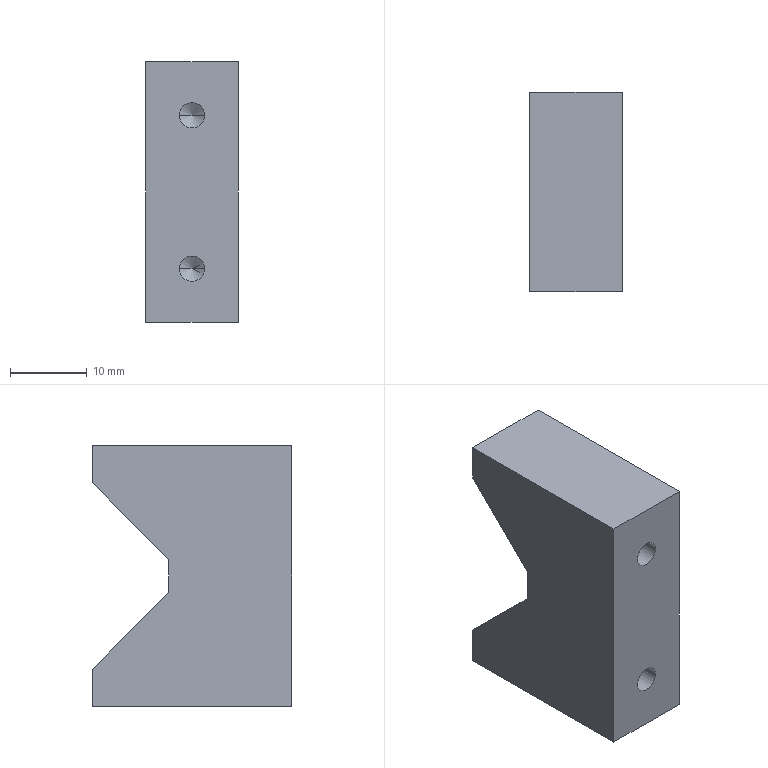Part | STEP file | 04-13 Guide block | 1 solid | 18 faces | box 12 x 26 x 34 mm | volume 8647 mm3 | plane 10 | cylinder 4 | cone 4 | commonest cylinder face diameters 3.3 x4
STEP:
#1=CARTESIAN_POINT('',(0.,0.,0.));
#2=DIRECTION('',(0.,0.,1.));
#3=DIRECTION('',(1.,0.,0.));
#4=AXIS2_PLACEMENT_3D('',#1,#2,#3);
#5=CARTESIAN_POINT('',(1.65,14.1,10.));
#6=VERTEX_POINT('',#5);
#7=CARTESIAN_POINT('',(1.65,0.,10.));
#8=VERTEX_POINT('',#7);
#9=CARTESIAN_POINT('',(1.65,14.1,10.));
#10=DIRECTION('',(0.,-1.,0.));
#11=VECTOR('',#10,1.);
#12=LINE('',#9,#11);
#13=CARTESIAN_POINT('',(0.,14.1,10.));
#14=DIRECTION('',(0.,-1.,0.));
#15=DIRECTION('',(1.,0.,0.));
#16=AXIS2_PLACEMENT_3D('',#13,#14,#15);
#17=CYLINDRICAL_SURFACE('',#16,1.65);
#18=CARTESIAN_POINT('',(6.283,0.));
#19=DIRECTION('',(0.,1.));
#20=VECTOR('',#19,1.);
#21=LINE('',#18,#20);
#22=(GEOMETRIC_REPRESENTATION_CONTEXT(2)PARAMETRIC_REPRESENTATION_CONTEXT()REPRESENTATION_CONTEXT('',''));
#23=DEFINITIONAL_REPRESENTATION('',(#21),#22);
#24=PCURVE('',#17,#23);
#25=CARTESIAN_POINT('',(0.,14.1,10.));
#26=DIRECTION('',(0.,-1.,0.));
#27=DIRECTION('',(1.,0.,0.));
#28=AXIS2_PLACEMENT_3D('',#25,#26,#27);
#29=CYLINDRICAL_SURFACE('',#28,1.65);
#30=CARTESIAN_POINT('',(0.,0.));
#31=DIRECTION('',(0.,1.));
#32=VECTOR('',#31,1.);
#33=LINE('',#30,#32);
#34=(GEOMETRIC_REPRESENTATION_CONTEXT(2)PARAMETRIC_REPRESENTATION_CONTEXT()REPRESENTATION_CONTEXT('',''));
#35=DEFINITIONAL_REPRESENTATION('',(#33),#34);
#36=PCURVE('',#29,#35);
#37=SURFACE_CURVE('',#12,(#24,#36),.PCURVE_S1.);
#38=EDGE_CURVE('',#6,#8,#37,.T.);
#39=ORIENTED_EDGE('',*,*,#38,.T.);
#40=CARTESIAN_POINT('',(-1.65,0.,10.));
#41=VERTEX_POINT('',#40);
#42=CARTESIAN_POINT('',(0.,0.,10.));
#43=DIRECTION('',(0.,-1.,0.));
#44=DIRECTION('',(1.,0.,0.));
#45=AXIS2_PLACEMENT_3D('',#42,#43,#44);
#46=CIRCLE('',#45,1.65);
#47=CARTESIAN_POINT('',(0.,14.1));
#48=DIRECTION('',(1.,0.));
#49=VECTOR('',#48,1.);
#50=LINE('',#47,#49);
#51=(GEOMETRIC_REPRESENTATION_CONTEXT(2)PARAMETRIC_REPRESENTATION_CONTEXT()REPRESENTATION_CONTEXT('',''));
#52=DEFINITIONAL_REPRESENTATION('',(#50),#51);
#53=PCURVE('',#17,#52);
#54=CARTESIAN_POINT('',(-6.,0.,-17.));
#55=DIRECTION('',(0.,1.,0.));
#56=DIRECTION('',(0.,0.,1.));
#57=AXIS2_PLACEMENT_3D('',#54,#55,#56);
#58=PLANE('',#57);
#59=CARTESIAN_POINT('',(27.,7.65));
#60=CARTESIAN_POINT('',(29.858,7.65));
#61=CARTESIAN_POINT('',(28.429,5.175));
#62=CARTESIAN_POINT('',(27.,2.7));
#63=CARTESIAN_POINT('',(25.571,5.175));
#64=CARTESIAN_POINT('',(24.142,7.65));
#65=CARTESIAN_POINT('',(27.,7.65));
#66=(BOUNDED_CURVE()B_SPLINE_CURVE(2,(#59,#60,#61,#62,#63,#64,#65),.UNSPECIFIED.,.T.,.F.)B_SPLINE_CURVE_WITH_KNOTS((1,2,2,2,2,1),(-2.094,0.,2.094,4.189,6.283,8.378),.UNSPECIFIED.)CURVE()GEOMETRIC_REPRESENTATION_ITEM()RATIONAL_B_SPLINE_CURVE((1.,0.5,1.,0.5,1.,0.5,1.))REPRESENTATION_ITEM(''));
#67=(GEOMETRIC_REPRESENTATION_CONTEXT(2)PARAMETRIC_REPRESENTATION_CONTEXT()REPRESENTATION_CONTEXT('',''));
#68=DEFINITIONAL_REPRESENTATION('',(#66),#67);
#69=PCURVE('',#58,#68);
#70=SURFACE_CURVE('',#46,(#53,#69),.PCURVE_S1.);
#71=EDGE_CURVE('',#41,#8,#70,.T.);
#72=ORIENTED_EDGE('',*,*,#71,.F.);
#73=CARTESIAN_POINT('',(-1.65,14.1,10.));
#74=VERTEX_POINT('',#73);
#75=CARTESIAN_POINT('',(-1.65,14.1,10.));
#76=DIRECTION('',(0.,-1.,0.));
#77=VECTOR('',#76,1.);
#78=LINE('',#75,#77);
#79=CARTESIAN_POINT('',(3.142,0.));
#80=DIRECTION('',(0.,1.));
#81=VECTOR('',#80,1.);
#82=LINE('',#79,#81);
#83=(GEOMETRIC_REPRESENTATION_CONTEXT(2)PARAMETRIC_REPRESENTATION_CONTEXT()REPRESENTATION_CONTEXT('',''));
#84=DEFINITIONAL_REPRESENTATION('',(#82),#83);
#85=PCURVE('',#17,#84);
#86=CARTESIAN_POINT('',(3.142,0.));
#87=DIRECTION('',(0.,1.));
#88=VECTOR('',#87,1.);
#89=LINE('',#86,#88);
#90=(GEOMETRIC_REPRESENTATION_CONTEXT(2)PARAMETRIC_REPRESENTATION_CONTEXT()REPRESENTATION_CONTEXT('',''));
#91=DEFINITIONAL_REPRESENTATION('',(#89),#90);
#92=PCURVE('',#29,#91);
#93=SURFACE_CURVE('',#78,(#85,#92),.PCURVE_S1.);
#94=EDGE_CURVE('',#74,#41,#93,.T.);
#95=ORIENTED_EDGE('',*,*,#94,.F.);
#96=CARTESIAN_POINT('',(0.,14.1,10.));
#97=DIRECTION('',(0.,1.,0.));
#98=DIRECTION('',(0.,0.,-1.));
#99=AXIS2_PLACEMENT_3D('',#96,#97,#98);
#100=CIRCLE('',#99,1.65);
#101=CARTESIAN_POINT('',(10.996,0.));
#102=DIRECTION('',(-1.,0.));
#103=VECTOR('',#102,1.);
#104=LINE('',#101,#103);
#105=(GEOMETRIC_REPRESENTATION_CONTEXT(2)PARAMETRIC_REPRESENTATION_CONTEXT()REPRESENTATION_CONTEXT('',''));
#106=DEFINITIONAL_REPRESENTATION('',(#104),#105);
#107=PCURVE('',#17,#106);
#108=CARTESIAN_POINT('',(0.,-984.909,10.));
#109=DIRECTION('',(0.,-1.,0.));
#110=DIRECTION('',(1.,0.,0.));
#111=AXIS2_PLACEMENT_3D('',#108,#109,#110);
#112=CONICAL_SURFACE('',#111,1664.279,1.03);
#113=CARTESIAN_POINT('',(10.996,-999.009));
#114=DIRECTION('',(-1.,0.));
#115=VECTOR('',#114,1.);
#116=LINE('',#113,#115);
#117=(GEOMETRIC_REPRESENTATION_CONTEXT(2)PARAMETRIC_REPRESENTATION_CONTEXT()REPRESENTATION_CONTEXT('',''));
#118=DEFINITIONAL_REPRESENTATION('',(#116),#117);
#119=PCURVE('',#112,#118);
#120=SURFACE_CURVE('',#100,(#107,#119),.PCURVE_S1.);
#121=EDGE_CURVE('',#6,#74,#120,.T.);
#122=ORIENTED_EDGE('',*,*,#121,.F.);
#123=EDGE_LOOP('',(#39,#72,#95,#122));
#124=FACE_BOUND('',#123,.F.);
#125=ADVANCED_FACE('',(#124),#17,.F.);
#126=ORIENTED_EDGE('',*,*,#121,.T.);
#127=CARTESIAN_POINT('',(0.,15.091,10.));
#128=VERTEX_POINT('',#127);
#129=CARTESIAN_POINT('',(0.,15.091,10.));
#130=DIRECTION('',(-0.8572,-0.515,0.));
#131=VECTOR('',#130,1.);
#132=LINE('',#129,#131);
#133=CARTESIAN_POINT('',(3.142,-1000.));
#134=CARTESIAN_POINT('',(3.142,-999.985));
#135=CARTESIAN_POINT('',(3.142,-999.955));
#136=CARTESIAN_POINT('',(3.142,-999.91));
#137=CARTESIAN_POINT('',(3.142,-999.865));
#138=CARTESIAN_POINT('',(3.142,-999.82));
#139=CARTESIAN_POINT('',(3.142,-999.775));
#140=CARTESIAN_POINT('',(3.142,-999.73));
#141=CARTESIAN_POINT('',(3.142,-999.685));
#142=CARTESIAN_POINT('',(3.142,-999.639));
#143=CARTESIAN_POINT('',(3.142,-999.594));
#144=CARTESIAN_POINT('',(3.142,-999.549));
#145=CARTESIAN_POINT('',(3.142,-999.504));
#146=CARTESIAN_POINT('',(3.142,-999.459));
#147=CARTESIAN_POINT('',(3.142,-999.414));
#148=CARTESIAN_POINT('',(3.142,-999.369));
#149=CARTESIAN_POINT('',(3.142,-999.324));
#150=CARTESIAN_POINT('',(3.142,-999.279));
#151=CARTESIAN_POINT('',(3.142,-999.234));
#152=CARTESIAN_POINT('',(3.142,-999.189));
#153=CARTESIAN_POINT('',(3.142,-999.144));
#154=CARTESIAN_POINT('',(3.142,-999.099));
#155=CARTESIAN_POINT('',(3.142,-999.054));
#156=CARTESIAN_POINT('',(3.142,-999.024));
#157=CARTESIAN_POINT('',(3.142,-999.009));
#158=B_SPLINE_CURVE_WITH_KNOTS('',3,(#133,#134,#135,#136,#137,#138,#139,#140,#141,#142,#143,#144,#145,#146,#147,#148,#149,#150,#151,#152,#153,#154,#155,#156,#157),.UNSPECIFIED.,.F.,.F.,(4,1,1,1,1,1,1,1,1,1,1,1,1,1,1,1,1,1,1,1,1,1,4),(0.,0.0875,0.175,0.2625,0.35,0.4375,0.525,0.6125,0.7,0.7875,0.875,0.9625,1.05,1.137,1.225,1.312,1.4,1.487,1.575,1.662,1.75,1.837,1.925),.QUASI_UNIFORM_KNOTS.);
#159=(GEOMETRIC_REPRESENTATION_CONTEXT(2)PARAMETRIC_REPRESENTATION_CONTEXT()REPRESENTATION_CONTEXT('',''));
#160=DEFINITIONAL_REPRESENTATION('',(#158),#159);
#161=PCURVE('',#112,#160);
#162=CARTESIAN_POINT('',(0.,-984.909,10.));
#163=DIRECTION('',(0.,-1.,0.));
#164=DIRECTION('',(1.,0.,0.));
#165=AXIS2_PLACEMENT_3D('',#162,#163,#164);
#166=CONICAL_SURFACE('',#165,1664.279,1.03);
#167=CARTESIAN_POINT('',(3.142,-1000.));
#168=CARTESIAN_POINT('',(3.142,-999.985));
#169=CARTESIAN_POINT('',(3.142,-999.955));
#170=CARTESIAN_POINT('',(3.142,-999.91));
#171=CARTESIAN_POINT('',(3.142,-999.865));
#172=CARTESIAN_POINT('',(3.142,-999.82));
#173=CARTESIAN_POINT('',(3.142,-999.775));
#174=CARTESIAN_POINT('',(3.142,-999.73));
#175=CARTESIAN_POINT('',(3.142,-999.685));
#176=CARTESIAN_POINT('',(3.142,-999.639));
#177=CARTESIAN_POINT('',(3.142,-999.594));
#178=CARTESIAN_POINT('',(3.142,-999.549));
#179=CARTESIAN_POINT('',(3.142,-999.504));
#180=CARTESIAN_POINT('',(3.142,-999.459));
#181=CARTESIAN_POINT('',(3.142,-999.414));
#182=CARTESIAN_POINT('',(3.142,-999.369));
#183=CARTESIAN_POINT('',(3.142,-999.324));
#184=CARTESIAN_POINT('',(3.142,-999.279));
#185=CARTESIAN_POINT('',(3.142,-999.234));
#186=CARTESIAN_POINT('',(3.142,-999.189));
#187=CARTESIAN_POINT('',(3.142,-999.144));
#188=CARTESIAN_POINT('',(3.142,-999.099));
#189=CARTESIAN_POINT('',(3.142,-999.054));
#190=CARTESIAN_POINT('',(3.142,-999.024));
#191=CARTESIAN_POINT('',(3.142,-999.009));
#192=B_SPLINE_CURVE_WITH_KNOTS('',3,(#167,#168,#169,#170,#171,#172,#173,#174,#175,#176,#177,#178,#179,#180,#181,#182,#183,#184,#185,#186,#187,#188,#189,#190,#191),.UNSPECIFIED.,.F.,.F.,(4,1,1,1,1,1,1,1,1,1,1,1,1,1,1,1,1,1,1,1,1,1,4),(0.,0.0875,0.175,0.2625,0.35,0.4375,0.525,0.6125,0.7,0.7875,0.875,0.9625,1.05,1.137,1.225,1.312,1.4,1.487,1.575,1.662,1.75,1.837,1.925),.QUASI_UNIFORM_KNOTS.);
#193=(GEOMETRIC_REPRESENTATION_CONTEXT(2)PARAMETRIC_REPRESENTATION_CONTEXT()REPRESENTATION_CONTEXT('',''));
#194=DEFINITIONAL_REPRESENTATION('',(#192),#193);
#195=PCURVE('',#166,#194);
#196=SURFACE_CURVE('',#132,(#161,#195),.PCURVE_S1.);
#197=EDGE_CURVE('',#128,#74,#196,.T.);
#198=ORIENTED_EDGE('',*,*,#197,.F.);
#199=CARTESIAN_POINT('',(0.,15.091,10.));
#200=DIRECTION('',(0.8572,-0.515,0.));
#201=VECTOR('',#200,1.);
#202=LINE('',#199,#201);
#203=CARTESIAN_POINT('',(6.283,-1000.));
#204=DIRECTION('',(0.,1.));
#205=VECTOR('',#204,1.);
#206=LINE('',#203,#205);
#207=(GEOMETRIC_REPRESENTATION_CONTEXT(2)PARAMETRIC_REPRESENTATION_CONTEXT()REPRESENTATION_CONTEXT('',''));
#208=DEFINITIONAL_REPRESENTATION('',(#206),#207);
#209=PCURVE('',#112,#208);
#210=CARTESIAN_POINT('',(0.,-1000.));
#211=DIRECTION('',(0.,1.));
#212=VECTOR('',#211,1.);
#213=LINE('',#210,#212);
#214=(GEOMETRIC_REPRESENTATION_CONTEXT(2)PARAMETRIC_REPRESENTATION_CONTEXT()REPRESENTATION_CONTEXT('',''));
#215=DEFINITIONAL_REPRESENTATION('',(#213),#214);
#216=PCURVE('',#166,#215);
#217=SURFACE_CURVE('',#202,(#209,#216),.PCURVE_S1.);
#218=EDGE_CURVE('',#128,#6,#217,.T.);
#219=ORIENTED_EDGE('',*,*,#218,.T.);
#220=EDGE_LOOP('',(#126,#198,#219));
#221=FACE_BOUND('',#220,.F.);
#222=ADVANCED_FACE('',(#221),#112,.F.);
#223=CARTESIAN_POINT('',(1.65,14.1,-10.));
#224=VERTEX_POINT('',#223);
#225=CARTESIAN_POINT('',(1.65,0.,-10.));
#226=VERTEX_POINT('',#225);
#227=CARTESIAN_POINT('',(1.65,14.1,-10.));
#228=DIRECTION('',(0.,-1.,0.));
#229=VECTOR('',#228,1.);
#230=LINE('',#227,#229);
#231=CARTESIAN_POINT('',(0.,14.1,-10.));
#232=DIRECTION('',(0.,-1.,0.));
#233=DIRECTION('',(1.,0.,0.));
#234=AXIS2_PLACEMENT_3D('',#231,#232,#233);
#235=CYLINDRICAL_SURFACE('',#234,1.65);
#236=CARTESIAN_POINT('',(6.283,0.));
#237=DIRECTION('',(0.,1.));
#238=VECTOR('',#237,1.);
#239=LINE('',#236,#238);
#240=(GEOMETRIC_REPRESENTATION_CONTEXT(2)PARAMETRIC_REPRESENTATION_CONTEXT()REPRESENTATION_CONTEXT('',''));
#241=DEFINITIONAL_REPRESENTATION('',(#239),#240);
#242=PCURVE('',#235,#241);
#243=CARTESIAN_POINT('',(0.,14.1,-10.));
#244=DIRECTION('',(0.,-1.,0.));
#245=DIRECTION('',(1.,0.,0.));
#246=AXIS2_PLACEMENT_3D('',#243,#244,#245);
#247=CYLINDRICAL_SURFACE('',#246,1.65);
#248=CARTESIAN_POINT('',(0.,0.));
#249=DIRECTION('',(0.,1.));
#250=VECTOR('',#249,1.);
#251=LINE('',#248,#250);
#252=(GEOMETRIC_REPRESENTATION_CONTEXT(2)PARAMETRIC_REPRESENTATION_CONTEXT()REPRESENTATION_CONTEXT('',''));
#253=DEFINITIONAL_REPRESENTATION('',(#251),#252);
#254=PCURVE('',#247,#253);
#255=SURFACE_CURVE('',#230,(#242,#254),.PCURVE_S1.);
#256=EDGE_CURVE('',#224,#226,#255,.T.);
#257=ORIENTED_EDGE('',*,*,#256,.T.);
#258=CARTESIAN_POINT('',(-1.65,0.,-10.));
#259=VERTEX_POINT('',#258);
#260=CARTESIAN_POINT('',(0.,0.,-10.));
#261=DIRECTION('',(0.,-1.,0.));
#262=DIRECTION('',(1.,0.,0.));
#263=AXIS2_PLACEMENT_3D('',#260,#261,#262);
#264=CIRCLE('',#263,1.65);
#265=CARTESIAN_POINT('',(0.,14.1));
#266=DIRECTION('',(1.,0.));
#267=VECTOR('',#266,1.);
#268=LINE('',#265,#267);
#269=(GEOMETRIC_REPRESENTATION_CONTEXT(2)PARAMETRIC_REPRESENTATION_CONTEXT()REPRESENTATION_CONTEXT('',''));
#270=DEFINITIONAL_REPRESENTATION('',(#268),#269);
#271=PCURVE('',#235,#270);
#272=CARTESIAN_POINT('',(7.,7.65));
#273=CARTESIAN_POINT('',(9.858,7.65));
#274=CARTESIAN_POINT('',(8.429,5.175));
#275=CARTESIAN_POINT('',(7.,2.7));
#276=CARTESIAN_POINT('',(5.571,5.175));
#277=CARTESIAN_POINT('',(4.142,7.65));
#278=CARTESIAN_POINT('',(7.,7.65));
#279=(BOUNDED_CURVE()B_SPLINE_CURVE(2,(#272,#273,#274,#275,#276,#277,#278),.UNSPECIFIED.,.T.,.F.)B_SPLINE_CURVE_WITH_KNOTS((1,2,2,2,2,1),(-2.094,0.,2.094,4.189,6.283,8.378),.UNSPECIFIED.)CURVE()GEOMETRIC_REPRESENTATION_ITEM()RATIONAL_B_SPLINE_CURVE((1.,0.5,1.,0.5,1.,0.5,1.))REPRESENTATION_ITEM(''));
#280=(GEOMETRIC_REPRESENTATION_CONTEXT(2)PARAMETRIC_REPRESENTATION_CONTEXT()REPRESENTATION_CONTEXT('',''));
#281=DEFINITIONAL_REPRESENTATION('',(#279),#280);
#282=PCURVE('',#58,#281);
#283=SURFACE_CURVE('',#264,(#271,#282),.PCURVE_S1.);
#284=EDGE_CURVE('',#259,#226,#283,.T.);
#285=ORIENTED_EDGE('',*,*,#284,.F.);
#286=CARTESIAN_POINT('',(-1.65,14.1,-10.));
#287=VERTEX_POINT('',#286);
#288=CARTESIAN_POINT('',(-1.65,14.1,-10.));
#289=DIRECTION('',(0.,-1.,0.));
#290=VECTOR('',#289,1.);
#291=LINE('',#288,#290);
#292=CARTESIAN_POINT('',(3.142,0.));
#293=DIRECTION('',(0.,1.));
#294=VECTOR('',#293,1.);
#295=LINE('',#292,#294);
#296=(GEOMETRIC_REPRESENTATION_CONTEXT(2)PARAMETRIC_REPRESENTATION_CONTEXT()REPRESENTATION_CONTEXT('',''));
#297=DEFINITIONAL_REPRESENTATION('',(#295),#296);
#298=PCURVE('',#235,#297);
#299=CARTESIAN_POINT('',(3.142,0.));
#300=DIRECTION('',(0.,1.));
#301=VECTOR('',#300,1.);
#302=LINE('',#299,#301);
#303=(GEOMETRIC_REPRESENTATION_CONTEXT(2)PARAMETRIC_REPRESENTATION_CONTEXT()REPRESENTATION_CONTEXT('',''));
#304=DEFINITIONAL_REPRESENTATION('',(#302),#303);
#305=PCURVE('',#247,#304);
#306=SURFACE_CURVE('',#291,(#298,#305),.PCURVE_S1.);
#307=EDGE_CURVE('',#287,#259,#306,.T.);
#308=ORIENTED_EDGE('',*,*,#307,.F.);
#309=CARTESIAN_POINT('',(0.,14.1,-10.));
#310=DIRECTION('',(0.,1.,0.));
#311=DIRECTION('',(0.,0.,-1.));
#312=AXIS2_PLACEMENT_3D('',#309,#310,#311);
#313=CIRCLE('',#312,1.65);
#314=CARTESIAN_POINT('',(10.996,0.));
#315=DIRECTION('',(-1.,0.));
#316=VECTOR('',#315,1.);
#317=LINE('',#314,#316);
#318=(GEOMETRIC_REPRESENTATION_CONTEXT(2)PARAMETRIC_REPRESENTATION_CONTEXT()REPRESENTATION_CONTEXT('',''));
#319=DEFINITIONAL_REPRESENTATION('',(#317),#318);
#320=PCURVE('',#235,#319);
#321=CARTESIAN_POINT('',(0.,-984.909,-10.));
#322=DIRECTION('',(0.,-1.,0.));
#323=DIRECTION('',(1.,0.,0.));
#324=AXIS2_PLACEMENT_3D('',#321,#322,#323);
#325=CONICAL_SURFACE('',#324,1664.279,1.03);
#326=CARTESIAN_POINT('',(10.996,-999.009));
#327=DIRECTION('',(-1.,0.));
#328=VECTOR('',#327,1.);
#329=LINE('',#326,#328);
#330=(GEOMETRIC_REPRESENTATION_CONTEXT(2)PARAMETRIC_REPRESENTATION_CONTEXT()REPRESENTATION_CONTEXT('',''));
#331=DEFINITIONAL_REPRESENTATION('',(#329),#330);
#332=PCURVE('',#325,#331);
#333=SURFACE_CURVE('',#313,(#320,#332),.PCURVE_S1.);
#334=EDGE_CURVE('',#224,#287,#333,.T.);
#335=ORIENTED_EDGE('',*,*,#334,.F.);
#336=EDGE_LOOP('',(#257,#285,#308,#335));
#337=FACE_BOUND('',#336,.F.);
#338=ADVANCED_FACE('',(#337),#235,.F.);
#339=ORIENTED_EDGE('',*,*,#334,.T.);
#340=CARTESIAN_POINT('',(0.,15.091,-10.));
#341=VERTEX_POINT('',#340);
#342=CARTESIAN_POINT('',(0.,15.091,-10.));
#343=DIRECTION('',(-0.8572,-0.515,0.));
#344=VECTOR('',#343,1.);
#345=LINE('',#342,#344);
#346=CARTESIAN_POINT('',(3.142,-1000.));
#347=CARTESIAN_POINT('',(3.142,-999.985));
#348=CARTESIAN_POINT('',(3.142,-999.955));
#349=CARTESIAN_POINT('',(3.142,-999.91));
#350=CARTESIAN_POINT('',(3.142,-999.865));
#351=CARTESIAN_POINT('',(3.142,-999.82));
#352=CARTESIAN_POINT('',(3.142,-999.775));
#353=CARTESIAN_POINT('',(3.142,-999.73));
#354=CARTESIAN_POINT('',(3.142,-999.685));
#355=CARTESIAN_POINT('',(3.142,-999.639));
#356=CARTESIAN_POINT('',(3.142,-999.594));
#357=CARTESIAN_POINT('',(3.142,-999.549));
#358=CARTESIAN_POINT('',(3.142,-999.504));
#359=CARTESIAN_POINT('',(3.142,-999.459));
#360=CARTESIAN_POINT('',(3.142,-999.414));
#361=CARTESIAN_POINT('',(3.142,-999.369));
#362=CARTESIAN_POINT('',(3.142,-999.324));
#363=CARTESIAN_POINT('',(3.142,-999.279));
#364=CARTESIAN_POINT('',(3.142,-999.234));
#365=CARTESIAN_POINT('',(3.142,-999.189));
#366=CARTESIAN_POINT('',(3.142,-999.144));
#367=CARTESIAN_POINT('',(3.142,-999.099));
#368=CARTESIAN_POINT('',(3.142,-999.054));
#369=CARTESIAN_POINT('',(3.142,-999.024));
#370=CARTESIAN_POINT('',(3.142,-999.009));
#371=B_SPLINE_CURVE_WITH_KNOTS('',3,(#346,#347,#348,#349,#350,#351,#352,#353,#354,#355,#356,#357,#358,#359,#360,#361,#362,#363,#364,#365,#366,#367,#368,#369,#370),.UNSPECIFIED.,.F.,.F.,(4,1,1,1,1,1,1,1,1,1,1,1,1,1,1,1,1,1,1,1,1,1,4),(0.,0.0875,0.175,0.2625,0.35,0.4375,0.525,0.6125,0.7,0.7875,0.875,0.9625,1.05,1.137,1.225,1.312,1.4,1.487,1.575,1.662,1.75,1.837,1.925),.QUASI_UNIFORM_KNOTS.);
#372=(GEOMETRIC_REPRESENTATION_CONTEXT(2)PARAMETRIC_REPRESENTATION_CONTEXT()REPRESENTATION_CONTEXT('',''));
#373=DEFINITIONAL_REPRESENTATION('',(#371),#372);
#374=PCURVE('',#325,#373);
#375=CARTESIAN_POINT('',(0.,-984.909,-10.));
#376=DIRECTION('',(0.,-1.,0.));
#377=DIRECTION('',(1.,0.,0.));
#378=AXIS2_PLACEMENT_3D('',#375,#376,#377);
#379=CONICAL_SURFACE('',#378,1664.279,1.03);
#380=CARTESIAN_POINT('',(3.142,-1000.));
#381=CARTESIAN_POINT('',(3.142,-999.985));
#382=CARTESIAN_POINT('',(3.142,-999.955));
#383=CARTESIAN_POINT('',(3.142,-999.91));
#384=CARTESIAN_POINT('',(3.142,-999.865));
#385=CARTESIAN_POINT('',(3.142,-999.82));
#386=CARTESIAN_POINT('',(3.142,-999.775));
#387=CARTESIAN_POINT('',(3.142,-999.73));
#388=CARTESIAN_POINT('',(3.142,-999.685));
#389=CARTESIAN_POINT('',(3.142,-999.639));
#390=CARTESIAN_POINT('',(3.142,-999.594));
#391=CARTESIAN_POINT('',(3.142,-999.549));
#392=CARTESIAN_POINT('',(3.142,-999.504));
#393=CARTESIAN_POINT('',(3.142,-999.459));
#394=CARTESIAN_POINT('',(3.142,-999.414));
#395=CARTESIAN_POINT('',(3.142,-999.369));
#396=CARTESIAN_POINT('',(3.142,-999.324));
#397=CARTESIAN_POINT('',(3.142,-999.279));
#398=CARTESIAN_POINT('',(3.142,-999.234));
#399=CARTESIAN_POINT('',(3.142,-999.189));
#400=CARTESIAN_POINT('',(3.142,-999.144));
#401=CARTESIAN_POINT('',(3.142,-999.099));
#402=CARTESIAN_POINT('',(3.142,-999.054));
#403=CARTESIAN_POINT('',(3.142,-999.024));
#404=CARTESIAN_POINT('',(3.142,-999.009));
#405=B_SPLINE_CURVE_WITH_KNOTS('',3,(#380,#381,#382,#383,#384,#385,#386,#387,#388,#389,#390,#391,#392,#393,#394,#395,#396,#397,#398,#399,#400,#401,#402,#403,#404),.UNSPECIFIED.,.F.,.F.,(4,1,1,1,1,1,1,1,1,1,1,1,1,1,1,1,1,1,1,1,1,1,4),(0.,0.0875,0.175,0.2625,0.35,0.4375,0.525,0.6125,0.7,0.7875,0.875,0.9625,1.05,1.137,1.225,1.312,1.4,1.487,1.575,1.662,1.75,1.837,1.925),.QUASI_UNIFORM_KNOTS.);
#406=(GEOMETRIC_REPRESENTATION_CONTEXT(2)PARAMETRIC_REPRESENTATION_CONTEXT()REPRESENTATION_CONTEXT('',''));
#407=DEFINITIONAL_REPRESENTATION('',(#405),#406);
#408=PCURVE('',#379,#407);
#409=SURFACE_CURVE('',#345,(#374,#408),.PCURVE_S1.);
#410=EDGE_CURVE('',#341,#287,#409,.T.);
#411=ORIENTED_EDGE('',*,*,#410,.F.);
#412=CARTESIAN_POINT('',(0.,15.091,-10.));
#413=DIRECTION('',(0.8572,-0.515,0.));
#414=VECTOR('',#413,1.);
#415=LINE('',#412,#414);
#416=CARTESIAN_POINT('',(6.283,-1000.));
#417=DIRECTION('',(0.,1.));
#418=VECTOR('',#417,1.);
#419=LINE('',#416,#418);
#420=(GEOMETRIC_REPRESENTATION_CONTEXT(2)PARAMETRIC_REPRESENTATION_CONTEXT()REPRESENTATION_CONTEXT('',''));
#421=DEFINITIONAL_REPRESENTATION('',(#419),#420);
#422=PCURVE('',#325,#421);
#423=CARTESIAN_POINT('',(0.,-1000.));
#424=DIRECTION('',(0.,1.));
#425=VECTOR('',#424,1.);
#426=LINE('',#423,#425);
#427=(GEOMETRIC_REPRESENTATION_CONTEXT(2)PARAMETRIC_REPRESENTATION_CONTEXT()REPRESENTATION_CONTEXT('',''));
#428=DEFINITIONAL_REPRESENTATION('',(#426),#427);
#429=PCURVE('',#379,#428);
#430=SURFACE_CURVE('',#415,(#422,#429),.PCURVE_S1.);
#431=EDGE_CURVE('',#341,#224,#430,.T.);
#432=ORIENTED_EDGE('',*,*,#431,.T.);
#433=EDGE_LOOP('',(#339,#411,#432));
#434=FACE_BOUND('',#433,.F.);
#435=ADVANCED_FACE('',(#434),#325,.F.);
#436=CARTESIAN_POINT('',(0.,0.,10.));
#437=DIRECTION('',(0.,-1.,0.));
#438=DIRECTION('',(1.,0.,0.));
#439=AXIS2_PLACEMENT_3D('',#436,#437,#438);
#440=CIRCLE('',#439,1.65);
#441=CARTESIAN_POINT('',(0.,14.1));
#442=DIRECTION('',(1.,0.));
#443=VECTOR('',#442,1.);
#444=LINE('',#441,#443);
#445=(GEOMETRIC_REPRESENTATION_CONTEXT(2)PARAMETRIC_REPRESENTATION_CONTEXT()REPRESENTATION_CONTEXT('',''));
#446=DEFINITIONAL_REPRESENTATION('',(#444),#445);
#447=PCURVE('',#29,#446);
#448=CARTESIAN_POINT('',(27.,7.65));
#449=CARTESIAN_POINT('',(29.858,7.65));
#450=CARTESIAN_POINT('',(28.429,5.175));
#451=CARTESIAN_POINT('',(27.,2.7));
#452=CARTESIAN_POINT('',(25.571,5.175));
#453=CARTESIAN_POINT('',(24.142,7.65));
#454=CARTESIAN_POINT('',(27.,7.65));
#455=(BOUNDED_CURVE()B_SPLINE_CURVE(2,(#448,#449,#450,#451,#452,#453,#454),.UNSPECIFIED.,.T.,.F.)B_SPLINE_CURVE_WITH_KNOTS((1,2,2,2,2,1),(-2.094,0.,2.094,4.189,6.283,8.378),.UNSPECIFIED.)CURVE()GEOMETRIC_REPRESENTATION_ITEM()RATIONAL_B_SPLINE_CURVE((1.,0.5,1.,0.5,1.,0.5,1.))REPRESENTATION_ITEM(''));
#456=(GEOMETRIC_REPRESENTATION_CONTEXT(2)PARAMETRIC_REPRESENTATION_CONTEXT()REPRESENTATION_CONTEXT('',''));
#457=DEFINITIONAL_REPRESENTATION('',(#455),#456);
#458=PCURVE('',#58,#457);
#459=SURFACE_CURVE('',#440,(#447,#458),.PCURVE_S1.);
#460=EDGE_CURVE('',#8,#41,#459,.T.);
#461=ORIENTED_EDGE('',*,*,#460,.F.);
#462=ORIENTED_EDGE('',*,*,#38,.F.);
#463=CARTESIAN_POINT('',(0.,14.1,10.));
#464=DIRECTION('',(0.,1.,0.));
#465=DIRECTION('',(0.,0.,-1.));
#466=AXIS2_PLACEMENT_3D('',#463,#464,#465);
#467=CIRCLE('',#466,1.65);
#468=CARTESIAN_POINT('',(4.712,0.));
#469=DIRECTION('',(-1.,0.));
#470=VECTOR('',#469,1.);
#471=LINE('',#468,#470);
#472=(GEOMETRIC_REPRESENTATION_CONTEXT(2)PARAMETRIC_REPRESENTATION_CONTEXT()REPRESENTATION_CONTEXT('',''));
#473=DEFINITIONAL_REPRESENTATION('',(#471),#472);
#474=PCURVE('',#29,#473);
#475=CARTESIAN_POINT('',(4.712,-999.009));
#476=DIRECTION('',(-1.,0.));
#477=VECTOR('',#476,1.);
#478=LINE('',#475,#477);
#479=(GEOMETRIC_REPRESENTATION_CONTEXT(2)PARAMETRIC_REPRESENTATION_CONTEXT()REPRESENTATION_CONTEXT('',''));
#480=DEFINITIONAL_REPRESENTATION('',(#478),#479);
#481=PCURVE('',#166,#480);
#482=SURFACE_CURVE('',#467,(#474,#481),.PCURVE_S1.);
#483=EDGE_CURVE('',#74,#6,#482,.T.);
#484=ORIENTED_EDGE('',*,*,#483,.F.);
#485=ORIENTED_EDGE('',*,*,#94,.T.);
#486=EDGE_LOOP('',(#461,#462,#484,#485));
#487=FACE_BOUND('',#486,.F.);
#488=ADVANCED_FACE('',(#487),#29,.F.);
#489=CARTESIAN_POINT('',(0.,0.,-10.));
#490=DIRECTION('',(0.,-1.,0.));
#491=DIRECTION('',(1.,0.,0.));
#492=AXIS2_PLACEMENT_3D('',#489,#490,#491);
#493=CIRCLE('',#492,1.65);
#494=CARTESIAN_POINT('',(7.,7.65));
#495=CARTESIAN_POINT('',(9.858,7.65));
#496=CARTESIAN_POINT('',(8.429,5.175));
#497=CARTESIAN_POINT('',(7.,2.7));
#498=CARTESIAN_POINT('',(5.571,5.175));
#499=CARTESIAN_POINT('',(4.142,7.65));
#500=CARTESIAN_POINT('',(7.,7.65));
#501=(BOUNDED_CURVE()B_SPLINE_CURVE(2,(#494,#495,#496,#497,#498,#499,#500),.UNSPECIFIED.,.T.,.F.)B_SPLINE_CURVE_WITH_KNOTS((1,2,2,2,2,1),(-2.094,0.,2.094,4.189,6.283,8.378),.UNSPECIFIED.)CURVE()GEOMETRIC_REPRESENTATION_ITEM()RATIONAL_B_SPLINE_CURVE((1.,0.5,1.,0.5,1.,0.5,1.))REPRESENTATION_ITEM(''));
#502=(GEOMETRIC_REPRESENTATION_CONTEXT(2)PARAMETRIC_REPRESENTATION_CONTEXT()REPRESENTATION_CONTEXT('',''));
#503=DEFINITIONAL_REPRESENTATION('',(#501),#502);
#504=PCURVE('',#58,#503);
#505=CARTESIAN_POINT('',(0.,14.1));
#506=DIRECTION('',(1.,0.));
#507=VECTOR('',#506,1.);
#508=LINE('',#505,#507);
#509=(GEOMETRIC_REPRESENTATION_CONTEXT(2)PARAMETRIC_REPRESENTATION_CONTEXT()REPRESENTATION_CONTEXT('',''));
#510=DEFINITIONAL_REPRESENTATION('',(#508),#509);
#511=PCURVE('',#247,#510);
#512=SURFACE_CURVE('',#493,(#504,#511),.PCURVE_S1.);
#513=EDGE_CURVE('',#226,#259,#512,.T.);
#514=ORIENTED_EDGE('',*,*,#513,.F.);
#515=ORIENTED_EDGE('',*,*,#284,.F.);
#516=EDGE_LOOP('',(#514,#515));
#517=FACE_BOUND('',#516,.T.);
#518=ORIENTED_EDGE('',*,*,#460,.F.);
#519=ORIENTED_EDGE('',*,*,#71,.F.);
#520=EDGE_LOOP('',(#518,#519));
#521=FACE_BOUND('',#520,.T.);
#522=CARTESIAN_POINT('',(6.,0.,-17.));
#523=VERTEX_POINT('',#522);
#524=CARTESIAN_POINT('',(-6.,0.,-17.));
#525=VERTEX_POINT('',#524);
#526=CARTESIAN_POINT('',(0.,0.,-17.));
#527=DIRECTION('',(-1.,0.,0.));
#528=VECTOR('',#527,1.);
#529=LINE('',#526,#528);
#530=CARTESIAN_POINT('',(0.,6.));
#531=DIRECTION('',(0.,-1.));
#532=VECTOR('',#531,1.);
#533=LINE('',#530,#532);
#534=(GEOMETRIC_REPRESENTATION_CONTEXT(2)PARAMETRIC_REPRESENTATION_CONTEXT()REPRESENTATION_CONTEXT('',''));
#535=DEFINITIONAL_REPRESENTATION('',(#533),#534);
#536=PCURVE('',#58,#535);
#537=CARTESIAN_POINT('',(-6.,0.,-17.));
#538=DIRECTION('',(0.,0.,1.));
#539=DIRECTION('',(1.,0.,0.));
#540=AXIS2_PLACEMENT_3D('',#537,#538,#539);
#541=PLANE('',#540);
#542=CARTESIAN_POINT('',(6.,0.));
#543=DIRECTION('',(-1.,0.));
#544=VECTOR('',#543,1.);
#545=LINE('',#542,#544);
#546=(GEOMETRIC_REPRESENTATION_CONTEXT(2)PARAMETRIC_REPRESENTATION_CONTEXT()REPRESENTATION_CONTEXT('',''));
#547=DEFINITIONAL_REPRESENTATION('',(#545),#546);
#548=PCURVE('',#541,#547);
#549=SURFACE_CURVE('',#529,(#536,#548),.PCURVE_S1.);
#550=EDGE_CURVE('',#523,#525,#549,.T.);
#551=ORIENTED_EDGE('',*,*,#550,.F.);
#552=CARTESIAN_POINT('',(6.,0.,17.));
#553=VERTEX_POINT('',#552);
#554=CARTESIAN_POINT('',(6.,0.,0.));
#555=DIRECTION('',(0.,0.,-1.));
#556=VECTOR('',#555,1.);
#557=LINE('',#554,#556);
#558=CARTESIAN_POINT('',(17.,12.));
#559=DIRECTION('',(-1.,0.));
#560=VECTOR('',#559,1.);
#561=LINE('',#558,#560);
#562=(GEOMETRIC_REPRESENTATION_CONTEXT(2)PARAMETRIC_REPRESENTATION_CONTEXT()REPRESENTATION_CONTEXT('',''));
#563=DEFINITIONAL_REPRESENTATION('',(#561),#562);
#564=PCURVE('',#58,#563);
#565=CARTESIAN_POINT('',(6.,0.,-17.));
#566=DIRECTION('',(-1.,0.,0.));
#567=DIRECTION('',(0.,0.,1.));
#568=AXIS2_PLACEMENT_3D('',#565,#566,#567);
#569=PLANE('',#568);
#570=CARTESIAN_POINT('',(17.,0.));
#571=DIRECTION('',(-1.,0.));
#572=VECTOR('',#571,1.);
#573=LINE('',#570,#572);
#574=(GEOMETRIC_REPRESENTATION_CONTEXT(2)PARAMETRIC_REPRESENTATION_CONTEXT()REPRESENTATION_CONTEXT('',''));
#575=DEFINITIONAL_REPRESENTATION('',(#573),#574);
#576=PCURVE('',#569,#575);
#577=SURFACE_CURVE('',#557,(#564,#576),.PCURVE_S1.);
#578=EDGE_CURVE('',#553,#523,#577,.T.);
#579=ORIENTED_EDGE('',*,*,#578,.F.);
#580=CARTESIAN_POINT('',(-6.,0.,17.));
#581=VERTEX_POINT('',#580);
#582=CARTESIAN_POINT('',(0.,0.,17.));
#583=DIRECTION('',(1.,0.,0.));
#584=VECTOR('',#583,1.);
#585=LINE('',#582,#584);
#586=CARTESIAN_POINT('',(34.,6.));
#587=DIRECTION('',(0.,1.));
#588=VECTOR('',#587,1.);
#589=LINE('',#586,#588);
#590=(GEOMETRIC_REPRESENTATION_CONTEXT(2)PARAMETRIC_REPRESENTATION_CONTEXT()REPRESENTATION_CONTEXT('',''));
#591=DEFINITIONAL_REPRESENTATION('',(#589),#590);
#592=PCURVE('',#58,#591);
#593=CARTESIAN_POINT('',(6.,0.,17.));
#594=DIRECTION('',(0.,0.,-1.));
#595=DIRECTION('',(-1.,0.,0.));
#596=AXIS2_PLACEMENT_3D('',#593,#594,#595);
#597=PLANE('',#596);
#598=CARTESIAN_POINT('',(6.,0.));
#599=DIRECTION('',(-1.,0.));
#600=VECTOR('',#599,1.);
#601=LINE('',#598,#600);
#602=(GEOMETRIC_REPRESENTATION_CONTEXT(2)PARAMETRIC_REPRESENTATION_CONTEXT()REPRESENTATION_CONTEXT('',''));
#603=DEFINITIONAL_REPRESENTATION('',(#601),#602);
#604=PCURVE('',#597,#603);
#605=SURFACE_CURVE('',#585,(#592,#604),.PCURVE_S1.);
#606=EDGE_CURVE('',#581,#553,#605,.T.);
#607=ORIENTED_EDGE('',*,*,#606,.F.);
#608=CARTESIAN_POINT('',(-6.,0.,0.));
#609=DIRECTION('',(0.,0.,1.));
#610=VECTOR('',#609,1.);
#611=LINE('',#608,#610);
#612=CARTESIAN_POINT('',(17.,0.));
#613=DIRECTION('',(1.,0.));
#614=VECTOR('',#613,1.);
#615=LINE('',#612,#614);
#616=(GEOMETRIC_REPRESENTATION_CONTEXT(2)PARAMETRIC_REPRESENTATION_CONTEXT()REPRESENTATION_CONTEXT('',''));
#617=DEFINITIONAL_REPRESENTATION('',(#615),#616);
#618=PCURVE('',#58,#617);
#619=CARTESIAN_POINT('',(-6.,0.,-17.));
#620=DIRECTION('',(-1.,0.,0.));
#621=DIRECTION('',(0.,0.,1.));
#622=AXIS2_PLACEMENT_3D('',#619,#620,#621);
#623=PLANE('',#622);
#624=CARTESIAN_POINT('',(17.,0.));
#625=DIRECTION('',(1.,0.));
#626=VECTOR('',#625,1.);
#627=LINE('',#624,#626);
#628=(GEOMETRIC_REPRESENTATION_CONTEXT(2)PARAMETRIC_REPRESENTATION_CONTEXT()REPRESENTATION_CONTEXT('',''));
#629=DEFINITIONAL_REPRESENTATION('',(#627),#628);
#630=PCURVE('',#623,#629);
#631=SURFACE_CURVE('',#611,(#618,#630),.PCURVE_S1.);
#632=EDGE_CURVE('',#525,#581,#631,.T.);
#633=ORIENTED_EDGE('',*,*,#632,.F.);
#634=EDGE_LOOP('',(#551,#579,#607,#633));
#635=FACE_BOUND('',#634,.T.);
#636=ADVANCED_FACE('',(#517,#521,#635),#58,.F.);
#637=ORIENTED_EDGE('',*,*,#483,.T.);
#638=ORIENTED_EDGE('',*,*,#218,.F.);
#639=ORIENTED_EDGE('',*,*,#197,.T.);
#640=EDGE_LOOP('',(#637,#638,#639));
#641=FACE_BOUND('',#640,.F.);
#642=ADVANCED_FACE('',(#641),#166,.F.);
#643=ORIENTED_EDGE('',*,*,#513,.F.);
#644=ORIENTED_EDGE('',*,*,#256,.F.);
#645=CARTESIAN_POINT('',(0.,14.1,-10.));
#646=DIRECTION('',(0.,1.,0.));
#647=DIRECTION('',(0.,0.,-1.));
#648=AXIS2_PLACEMENT_3D('',#645,#646,#647);
#649=CIRCLE('',#648,1.65);
#650=CARTESIAN_POINT('',(4.712,0.));
#651=DIRECTION('',(-1.,0.));
#652=VECTOR('',#651,1.);
#653=LINE('',#650,#652);
#654=(GEOMETRIC_REPRESENTATION_CONTEXT(2)PARAMETRIC_REPRESENTATION_CONTEXT()REPRESENTATION_CONTEXT('',''));
#655=DEFINITIONAL_REPRESENTATION('',(#653),#654);
#656=PCURVE('',#247,#655);
#657=CARTESIAN_POINT('',(4.712,-999.009));
#658=DIRECTION('',(-1.,0.));
#659=VECTOR('',#658,1.);
#660=LINE('',#657,#659);
#661=(GEOMETRIC_REPRESENTATION_CONTEXT(2)PARAMETRIC_REPRESENTATION_CONTEXT()REPRESENTATION_CONTEXT('',''));
#662=DEFINITIONAL_REPRESENTATION('',(#660),#661);
#663=PCURVE('',#379,#662);
#664=SURFACE_CURVE('',#649,(#656,#663),.PCURVE_S1.);
#665=EDGE_CURVE('',#287,#224,#664,.T.);
#666=ORIENTED_EDGE('',*,*,#665,.F.);
#667=ORIENTED_EDGE('',*,*,#307,.T.);
#668=EDGE_LOOP('',(#643,#644,#666,#667));
#669=FACE_BOUND('',#668,.F.);
#670=ADVANCED_FACE('',(#669),#247,.F.);
#671=CARTESIAN_POINT('',(-6.,26.,-17.));
#672=VERTEX_POINT('',#671);
#673=CARTESIAN_POINT('',(-6.,13.,-17.));
#674=DIRECTION('',(0.,-1.,0.));
#675=VECTOR('',#674,1.);
#676=LINE('',#673,#675);
#677=CARTESIAN_POINT('',(0.,13.));
#678=DIRECTION('',(0.,-1.));
#679=VECTOR('',#678,1.);
#680=LINE('',#677,#679);
#681=(GEOMETRIC_REPRESENTATION_CONTEXT(2)PARAMETRIC_REPRESENTATION_CONTEXT()REPRESENTATION_CONTEXT('',''));
#682=DEFINITIONAL_REPRESENTATION('',(#680),#681);
#683=PCURVE('',#623,#682);
#684=CARTESIAN_POINT('',(0.,13.));
#685=DIRECTION('',(0.,-1.));
#686=VECTOR('',#685,1.);
#687=LINE('',#684,#686);
#688=(GEOMETRIC_REPRESENTATION_CONTEXT(2)PARAMETRIC_REPRESENTATION_CONTEXT()REPRESENTATION_CONTEXT('',''));
#689=DEFINITIONAL_REPRESENTATION('',(#687),#688);
#690=PCURVE('',#541,#689);
#691=SURFACE_CURVE('',#676,(#683,#690),.PCURVE_S1.);
#692=EDGE_CURVE('',#672,#525,#691,.T.);
#693=ORIENTED_EDGE('',*,*,#692,.T.);
#694=ORIENTED_EDGE('',*,*,#632,.T.);
#695=CARTESIAN_POINT('',(-6.,26.,17.));
#696=VERTEX_POINT('',#695);
#697=CARTESIAN_POINT('',(-6.,13.,17.));
#698=DIRECTION('',(0.,1.,0.));
#699=VECTOR('',#698,1.);
#700=LINE('',#697,#699);
#701=CARTESIAN_POINT('',(34.,13.));
#702=DIRECTION('',(0.,1.));
#703=VECTOR('',#702,1.);
#704=LINE('',#701,#703);
#705=(GEOMETRIC_REPRESENTATION_CONTEXT(2)PARAMETRIC_REPRESENTATION_CONTEXT()REPRESENTATION_CONTEXT('',''));
#706=DEFINITIONAL_REPRESENTATION('',(#704),#705);
#707=PCURVE('',#623,#706);
#708=CARTESIAN_POINT('',(12.,13.));
#709=DIRECTION('',(0.,1.));
#710=VECTOR('',#709,1.);
#711=LINE('',#708,#710);
#712=(GEOMETRIC_REPRESENTATION_CONTEXT(2)PARAMETRIC_REPRESENTATION_CONTEXT()REPRESENTATION_CONTEXT('',''));
#713=DEFINITIONAL_REPRESENTATION('',(#711),#712);
#714=PCURVE('',#597,#713);
#715=SURFACE_CURVE('',#700,(#707,#714),.PCURVE_S1.);
#716=EDGE_CURVE('',#581,#696,#715,.T.);
#717=ORIENTED_EDGE('',*,*,#716,.T.);
#718=CARTESIAN_POINT('',(-6.,26.,12.142));
#719=VERTEX_POINT('',#718);
#720=CARTESIAN_POINT('',(-6.,26.,0.));
#721=DIRECTION('',(0.,0.,-1.));
#722=VECTOR('',#721,1.);
#723=LINE('',#720,#722);
#724=CARTESIAN_POINT('',(17.,26.));
#725=DIRECTION('',(-1.,0.));
#726=VECTOR('',#725,1.);
#727=LINE('',#724,#726);
#728=(GEOMETRIC_REPRESENTATION_CONTEXT(2)PARAMETRIC_REPRESENTATION_CONTEXT()REPRESENTATION_CONTEXT('',''));
#729=DEFINITIONAL_REPRESENTATION('',(#727),#728);
#730=PCURVE('',#623,#729);
#731=CARTESIAN_POINT('',(-6.,26.,17.));
#732=DIRECTION('',(0.,-1.,0.));
#733=DIRECTION('',(0.,0.,-1.));
#734=AXIS2_PLACEMENT_3D('',#731,#732,#733);
#735=PLANE('',#734);
#736=CARTESIAN_POINT('',(17.,0.));
#737=DIRECTION('',(1.,0.));
#738=VECTOR('',#737,1.);
#739=LINE('',#736,#738);
#740=(GEOMETRIC_REPRESENTATION_CONTEXT(2)PARAMETRIC_REPRESENTATION_CONTEXT()REPRESENTATION_CONTEXT('',''));
#741=DEFINITIONAL_REPRESENTATION('',(#739),#740);
#742=PCURVE('',#735,#741);
#743=SURFACE_CURVE('',#723,(#730,#742),.PCURVE_S1.);
#744=EDGE_CURVE('',#696,#719,#743,.T.);
#745=ORIENTED_EDGE('',*,*,#744,.T.);
#746=CARTESIAN_POINT('',(-6.,16.,2.142));
#747=VERTEX_POINT('',#746);
#748=CARTESIAN_POINT('',(-6.,26.,12.142));
#749=DIRECTION('',(0.,-0.7071,-0.7071));
#750=VECTOR('',#749,1.);
#751=LINE('',#748,#750);
#752=CARTESIAN_POINT('',(29.142,26.));
#753=DIRECTION('',(-0.7071,-0.7071));
#754=VECTOR('',#753,1.);
#755=LINE('',#752,#754);
#756=(GEOMETRIC_REPRESENTATION_CONTEXT(2)PARAMETRIC_REPRESENTATION_CONTEXT()REPRESENTATION_CONTEXT('',''));
#757=DEFINITIONAL_REPRESENTATION('',(#755),#756);
#758=PCURVE('',#623,#757);
#759=CARTESIAN_POINT('',(-6.,26.,12.142));
#760=DIRECTION('',(0.,-0.7071,0.7071));
#761=DIRECTION('',(0.,-0.7071,-0.7071));
#762=AXIS2_PLACEMENT_3D('',#759,#760,#761);
#763=PLANE('',#762);
#764=CARTESIAN_POINT('',(0.,0.));
#765=DIRECTION('',(1.,0.));
#766=VECTOR('',#765,1.);
#767=LINE('',#764,#766);
#768=(GEOMETRIC_REPRESENTATION_CONTEXT(2)PARAMETRIC_REPRESENTATION_CONTEXT()REPRESENTATION_CONTEXT('',''));
#769=DEFINITIONAL_REPRESENTATION('',(#767),#768);
#770=PCURVE('',#763,#769);
#771=SURFACE_CURVE('',#751,(#758,#770),.PCURVE_S1.);
#772=EDGE_CURVE('',#719,#747,#771,.T.);
#773=ORIENTED_EDGE('',*,*,#772,.T.);
#774=CARTESIAN_POINT('',(-6.,16.,-2.142));
#775=VERTEX_POINT('',#774);
#776=CARTESIAN_POINT('',(-6.,16.,0.));
#777=DIRECTION('',(0.,0.,-1.));
#778=VECTOR('',#777,1.);
#779=LINE('',#776,#778);
#780=CARTESIAN_POINT('',(17.,16.));
#781=DIRECTION('',(-1.,0.));
#782=VECTOR('',#781,1.);
#783=LINE('',#780,#782);
#784=(GEOMETRIC_REPRESENTATION_CONTEXT(2)PARAMETRIC_REPRESENTATION_CONTEXT()REPRESENTATION_CONTEXT('',''));
#785=DEFINITIONAL_REPRESENTATION('',(#783),#784);
#786=PCURVE('',#623,#785);
#787=CARTESIAN_POINT('',(-6.,16.,2.142));
#788=DIRECTION('',(0.,-1.,0.));
#789=DIRECTION('',(0.,0.,-1.));
#790=AXIS2_PLACEMENT_3D('',#787,#788,#789);
#791=PLANE('',#790);
#792=CARTESIAN_POINT('',(2.142,0.));
#793=DIRECTION('',(1.,0.));
#794=VECTOR('',#793,1.);
#795=LINE('',#792,#794);
#796=(GEOMETRIC_REPRESENTATION_CONTEXT(2)PARAMETRIC_REPRESENTATION_CONTEXT()REPRESENTATION_CONTEXT('',''));
#797=DEFINITIONAL_REPRESENTATION('',(#795),#796);
#798=PCURVE('',#791,#797);
#799=SURFACE_CURVE('',#779,(#786,#798),.PCURVE_S1.);
#800=EDGE_CURVE('',#747,#775,#799,.T.);
#801=ORIENTED_EDGE('',*,*,#800,.T.);
#802=CARTESIAN_POINT('',(-6.,26.,-12.142));
#803=VERTEX_POINT('',#802);
#804=CARTESIAN_POINT('',(-6.,16.,-2.142));
#805=DIRECTION('',(0.,0.7071,-0.7071));
#806=VECTOR('',#805,1.);
#807=LINE('',#804,#806);
#808=CARTESIAN_POINT('',(14.858,16.));
#809=DIRECTION('',(-0.7071,0.7071));
#810=VECTOR('',#809,1.);
#811=LINE('',#808,#810);
#812=(GEOMETRIC_REPRESENTATION_CONTEXT(2)PARAMETRIC_REPRESENTATION_CONTEXT()REPRESENTATION_CONTEXT('',''));
#813=DEFINITIONAL_REPRESENTATION('',(#811),#812);
#814=PCURVE('',#623,#813);
#815=CARTESIAN_POINT('',(-6.,16.,-2.142));
#816=DIRECTION('',(0.,-0.7071,-0.7071));
#817=DIRECTION('',(0.,0.7071,-0.7071));
#818=AXIS2_PLACEMENT_3D('',#815,#816,#817);
#819=PLANE('',#818);
#820=CARTESIAN_POINT('',(-0.000000006,0.));
#821=DIRECTION('',(1.,0.));
#822=VECTOR('',#821,1.);
#823=LINE('',#820,#822);
#824=(GEOMETRIC_REPRESENTATION_CONTEXT(2)PARAMETRIC_REPRESENTATION_CONTEXT()REPRESENTATION_CONTEXT('',''));
#825=DEFINITIONAL_REPRESENTATION('',(#823),#824);
#826=PCURVE('',#819,#825);
#827=SURFACE_CURVE('',#807,(#814,#826),.PCURVE_S1.);
#828=EDGE_CURVE('',#775,#803,#827,.T.);
#829=ORIENTED_EDGE('',*,*,#828,.T.);
#830=CARTESIAN_POINT('',(-6.,26.,0.));
#831=DIRECTION('',(0.,0.,-1.));
#832=VECTOR('',#831,1.);
#833=LINE('',#830,#832);
#834=CARTESIAN_POINT('',(17.,26.));
#835=DIRECTION('',(-1.,0.));
#836=VECTOR('',#835,1.);
#837=LINE('',#834,#836);
#838=(GEOMETRIC_REPRESENTATION_CONTEXT(2)PARAMETRIC_REPRESENTATION_CONTEXT()REPRESENTATION_CONTEXT('',''));
#839=DEFINITIONAL_REPRESENTATION('',(#837),#838);
#840=PCURVE('',#623,#839);
#841=CARTESIAN_POINT('',(-6.,26.,-12.142));
#842=DIRECTION('',(0.,-1.,0.));
#843=DIRECTION('',(0.,0.,-1.));
#844=AXIS2_PLACEMENT_3D('',#841,#842,#843);
#845=PLANE('',#844);
#846=CARTESIAN_POINT('',(-12.142,0.));
#847=DIRECTION('',(1.,0.));
#848=VECTOR('',#847,1.);
#849=LINE('',#846,#848);
#850=(GEOMETRIC_REPRESENTATION_CONTEXT(2)PARAMETRIC_REPRESENTATION_CONTEXT()REPRESENTATION_CONTEXT('',''));
#851=DEFINITIONAL_REPRESENTATION('',(#849),#850);
#852=PCURVE('',#845,#851);
#853=SURFACE_CURVE('',#833,(#840,#852),.PCURVE_S1.);
#854=EDGE_CURVE('',#803,#672,#853,.T.);
#855=ORIENTED_EDGE('',*,*,#854,.T.);
#856=EDGE_LOOP('',(#693,#694,#717,#745,#773,#801,#829,#855));
#857=FACE_BOUND('',#856,.T.);
#858=ADVANCED_FACE('',(#857),#623,.T.);
#859=CARTESIAN_POINT('',(6.,26.,-17.));
#860=VERTEX_POINT('',#859);
#861=CARTESIAN_POINT('',(0.,26.,-17.));
#862=DIRECTION('',(-1.,0.,0.));
#863=VECTOR('',#862,1.);
#864=LINE('',#861,#863);
#865=CARTESIAN_POINT('',(6.,26.));
#866=DIRECTION('',(-1.,0.));
#867=VECTOR('',#866,1.);
#868=LINE('',#865,#867);
#869=(GEOMETRIC_REPRESENTATION_CONTEXT(2)PARAMETRIC_REPRESENTATION_CONTEXT()REPRESENTATION_CONTEXT('',''));
#870=DEFINITIONAL_REPRESENTATION('',(#868),#869);
#871=PCURVE('',#541,#870);
#872=CARTESIAN_POINT('',(4.858,6.));
#873=DIRECTION('',(0.,-1.));
#874=VECTOR('',#873,1.);
#875=LINE('',#872,#874);
#876=(GEOMETRIC_REPRESENTATION_CONTEXT(2)PARAMETRIC_REPRESENTATION_CONTEXT()REPRESENTATION_CONTEXT('',''));
#877=DEFINITIONAL_REPRESENTATION('',(#875),#876);
#878=PCURVE('',#845,#877);
#879=SURFACE_CURVE('',#864,(#871,#878),.PCURVE_S1.);
#880=EDGE_CURVE('',#860,#672,#879,.T.);
#881=ORIENTED_EDGE('',*,*,#880,.F.);
#882=CARTESIAN_POINT('',(6.,13.,-17.));
#883=DIRECTION('',(0.,1.,0.));
#884=VECTOR('',#883,1.);
#885=LINE('',#882,#884);
#886=CARTESIAN_POINT('',(12.,13.));
#887=DIRECTION('',(0.,1.));
#888=VECTOR('',#887,1.);
#889=LINE('',#886,#888);
#890=(GEOMETRIC_REPRESENTATION_CONTEXT(2)PARAMETRIC_REPRESENTATION_CONTEXT()REPRESENTATION_CONTEXT('',''));
#891=DEFINITIONAL_REPRESENTATION('',(#889),#890);
#892=PCURVE('',#541,#891);
#893=CARTESIAN_POINT('',(0.,13.));
#894=DIRECTION('',(0.,1.));
#895=VECTOR('',#894,1.);
#896=LINE('',#893,#895);
#897=(GEOMETRIC_REPRESENTATION_CONTEXT(2)PARAMETRIC_REPRESENTATION_CONTEXT()REPRESENTATION_CONTEXT('',''));
#898=DEFINITIONAL_REPRESENTATION('',(#896),#897);
#899=PCURVE('',#569,#898);
#900=SURFACE_CURVE('',#885,(#892,#899),.PCURVE_S1.);
#901=EDGE_CURVE('',#523,#860,#900,.T.);
#902=ORIENTED_EDGE('',*,*,#901,.F.);
#903=ORIENTED_EDGE('',*,*,#550,.T.);
#904=ORIENTED_EDGE('',*,*,#692,.F.);
#905=EDGE_LOOP('',(#881,#902,#903,#904));
#906=FACE_BOUND('',#905,.T.);
#907=ADVANCED_FACE('',(#906),#541,.F.);
#908=ORIENTED_EDGE('',*,*,#578,.T.);
#909=ORIENTED_EDGE('',*,*,#901,.T.);
#910=CARTESIAN_POINT('',(6.,26.,-12.142));
#911=VERTEX_POINT('',#910);
#912=CARTESIAN_POINT('',(6.,26.,0.));
#913=DIRECTION('',(0.,0.,-1.));
#914=VECTOR('',#913,1.);
#915=LINE('',#912,#914);
#916=CARTESIAN_POINT('',(17.,26.));
#917=DIRECTION('',(-1.,0.));
#918=VECTOR('',#917,1.);
#919=LINE('',#916,#918);
#920=(GEOMETRIC_REPRESENTATION_CONTEXT(2)PARAMETRIC_REPRESENTATION_CONTEXT()REPRESENTATION_CONTEXT('',''));
#921=DEFINITIONAL_REPRESENTATION('',(#919),#920);
#922=PCURVE('',#569,#921);
#923=CARTESIAN_POINT('',(-12.142,12.));
#924=DIRECTION('',(1.,0.));
#925=VECTOR('',#924,1.);
#926=LINE('',#923,#925);
#927=(GEOMETRIC_REPRESENTATION_CONTEXT(2)PARAMETRIC_REPRESENTATION_CONTEXT()REPRESENTATION_CONTEXT('',''));
#928=DEFINITIONAL_REPRESENTATION('',(#926),#927);
#929=PCURVE('',#845,#928);
#930=SURFACE_CURVE('',#915,(#922,#929),.PCURVE_S1.);
#931=EDGE_CURVE('',#911,#860,#930,.T.);
#932=ORIENTED_EDGE('',*,*,#931,.F.);
#933=CARTESIAN_POINT('',(6.,16.,-2.142));
#934=VERTEX_POINT('',#933);
#935=CARTESIAN_POINT('',(6.,16.,-2.142));
#936=DIRECTION('',(0.,0.7071,-0.7071));
#937=VECTOR('',#936,1.);
#938=LINE('',#935,#937);
#939=CARTESIAN_POINT('',(14.858,16.));
#940=DIRECTION('',(-0.7071,0.7071));
#941=VECTOR('',#940,1.);
#942=LINE('',#939,#941);
#943=(GEOMETRIC_REPRESENTATION_CONTEXT(2)PARAMETRIC_REPRESENTATION_CONTEXT()REPRESENTATION_CONTEXT('',''));
#944=DEFINITIONAL_REPRESENTATION('',(#942),#943);
#945=PCURVE('',#569,#944);
#946=CARTESIAN_POINT('',(0.,12.));
#947=DIRECTION('',(1.,0.));
#948=VECTOR('',#947,1.);
#949=LINE('',#946,#948);
#950=(GEOMETRIC_REPRESENTATION_CONTEXT(2)PARAMETRIC_REPRESENTATION_CONTEXT()REPRESENTATION_CONTEXT('',''));
#951=DEFINITIONAL_REPRESENTATION('',(#949),#950);
#952=PCURVE('',#819,#951);
#953=SURFACE_CURVE('',#938,(#945,#952),.PCURVE_S1.);
#954=EDGE_CURVE('',#934,#911,#953,.T.);
#955=ORIENTED_EDGE('',*,*,#954,.F.);
#956=CARTESIAN_POINT('',(6.,16.,2.142));
#957=VERTEX_POINT('',#956);
#958=CARTESIAN_POINT('',(6.,16.,0.));
#959=DIRECTION('',(0.,0.,-1.));
#960=VECTOR('',#959,1.);
#961=LINE('',#958,#960);
#962=CARTESIAN_POINT('',(17.,16.));
#963=DIRECTION('',(-1.,0.));
#964=VECTOR('',#963,1.);
#965=LINE('',#962,#964);
#966=(GEOMETRIC_REPRESENTATION_CONTEXT(2)PARAMETRIC_REPRESENTATION_CONTEXT()REPRESENTATION_CONTEXT('',''));
#967=DEFINITIONAL_REPRESENTATION('',(#965),#966);
#968=PCURVE('',#569,#967);
#969=CARTESIAN_POINT('',(2.142,12.));
#970=DIRECTION('',(1.,0.));
#971=VECTOR('',#970,1.);
#972=LINE('',#969,#971);
#973=(GEOMETRIC_REPRESENTATION_CONTEXT(2)PARAMETRIC_REPRESENTATION_CONTEXT()REPRESENTATION_CONTEXT('',''));
#974=DEFINITIONAL_REPRESENTATION('',(#972),#973);
#975=PCURVE('',#791,#974);
#976=SURFACE_CURVE('',#961,(#968,#975),.PCURVE_S1.);
#977=EDGE_CURVE('',#957,#934,#976,.T.);
#978=ORIENTED_EDGE('',*,*,#977,.F.);
#979=CARTESIAN_POINT('',(6.,26.,12.142));
#980=VERTEX_POINT('',#979);
#981=CARTESIAN_POINT('',(6.,26.,12.142));
#982=DIRECTION('',(0.,-0.7071,-0.7071));
#983=VECTOR('',#982,1.);
#984=LINE('',#981,#983);
#985=CARTESIAN_POINT('',(29.142,26.));
#986=DIRECTION('',(-0.7071,-0.7071));
#987=VECTOR('',#986,1.);
#988=LINE('',#985,#987);
#989=(GEOMETRIC_REPRESENTATION_CONTEXT(2)PARAMETRIC_REPRESENTATION_CONTEXT()REPRESENTATION_CONTEXT('',''));
#990=DEFINITIONAL_REPRESENTATION('',(#988),#989);
#991=PCURVE('',#569,#990);
#992=CARTESIAN_POINT('',(0.,12.));
#993=DIRECTION('',(1.,0.));
#994=VECTOR('',#993,1.);
#995=LINE('',#992,#994);
#996=(GEOMETRIC_REPRESENTATION_CONTEXT(2)PARAMETRIC_REPRESENTATION_CONTEXT()REPRESENTATION_CONTEXT('',''));
#997=DEFINITIONAL_REPRESENTATION('',(#995),#996);
#998=PCURVE('',#763,#997);
#999=SURFACE_CURVE('',#984,(#991,#998),.PCURVE_S1.);
#1000=EDGE_CURVE('',#980,#957,#999,.T.);
#1001=ORIENTED_EDGE('',*,*,#1000,.F.);
#1002=CARTESIAN_POINT('',(6.,26.,17.));
#1003=VERTEX_POINT('',#1002);
#1004=CARTESIAN_POINT('',(6.,26.,0.));
#1005=DIRECTION('',(0.,0.,-1.));
#1006=VECTOR('',#1005,1.);
#1007=LINE('',#1004,#1006);
#1008=CARTESIAN_POINT('',(17.,26.));
#1009=DIRECTION('',(-1.,0.));
#1010=VECTOR('',#1009,1.);
#1011=LINE('',#1008,#1010);
#1012=(GEOMETRIC_REPRESENTATION_CONTEXT(2)PARAMETRIC_REPRESENTATION_CONTEXT()REPRESENTATION_CONTEXT('',''));
#1013=DEFINITIONAL_REPRESENTATION('',(#1011),#1012);
#1014=PCURVE('',#569,#1013);
#1015=CARTESIAN_POINT('',(17.,12.));
#1016=DIRECTION('',(1.,0.));
#1017=VECTOR('',#1016,1.);
#1018=LINE('',#1015,#1017);
#1019=(GEOMETRIC_REPRESENTATION_CONTEXT(2)PARAMETRIC_REPRESENTATION_CONTEXT()REPRESENTATION_CONTEXT('',''));
#1020=DEFINITIONAL_REPRESENTATION('',(#1018),#1019);
#1021=PCURVE('',#735,#1020);
#1022=SURFACE_CURVE('',#1007,(#1014,#1021),.PCURVE_S1.);
#1023=EDGE_CURVE('',#1003,#980,#1022,.T.);
#1024=ORIENTED_EDGE('',*,*,#1023,.F.);
#1025=CARTESIAN_POINT('',(6.,13.,17.));
#1026=DIRECTION('',(0.,1.,0.));
#1027=VECTOR('',#1026,1.);
#1028=LINE('',#1025,#1027);
#1029=CARTESIAN_POINT('',(34.,13.));
#1030=DIRECTION('',(0.,1.));
#1031=VECTOR('',#1030,1.);
#1032=LINE('',#1029,#1031);
#1033=(GEOMETRIC_REPRESENTATION_CONTEXT(2)PARAMETRIC_REPRESENTATION_CONTEXT()REPRESENTATION_CONTEXT('',''));
#1034=DEFINITIONAL_REPRESENTATION('',(#1032),#1033);
#1035=PCURVE('',#569,#1034);
#1036=CARTESIAN_POINT('',(0.,13.));
#1037=DIRECTION('',(0.,1.));
#1038=VECTOR('',#1037,1.);
#1039=LINE('',#1036,#1038);
#1040=(GEOMETRIC_REPRESENTATION_CONTEXT(2)PARAMETRIC_REPRESENTATION_CONTEXT()REPRESENTATION_CONTEXT('',''));
#1041=DEFINITIONAL_REPRESENTATION('',(#1039),#1040);
#1042=PCURVE('',#597,#1041);
#1043=SURFACE_CURVE('',#1028,(#1035,#1042),.PCURVE_S1.);
#1044=EDGE_CURVE('',#553,#1003,#1043,.T.);
#1045=ORIENTED_EDGE('',*,*,#1044,.F.);
#1046=EDGE_LOOP('',(#908,#909,#932,#955,#978,#1001,#1024,#1045));
#1047=FACE_BOUND('',#1046,.T.);
#1048=ADVANCED_FACE('',(#1047),#569,.F.);
#1049=ORIENTED_EDGE('',*,*,#606,.T.);
#1050=ORIENTED_EDGE('',*,*,#1044,.T.);
#1051=CARTESIAN_POINT('',(0.,26.,17.));
#1052=DIRECTION('',(1.,0.,0.));
#1053=VECTOR('',#1052,1.);
#1054=LINE('',#1051,#1053);
#1055=CARTESIAN_POINT('',(6.,26.));
#1056=DIRECTION('',(-1.,0.));
#1057=VECTOR('',#1056,1.);
#1058=LINE('',#1055,#1057);
#1059=(GEOMETRIC_REPRESENTATION_CONTEXT(2)PARAMETRIC_REPRESENTATION_CONTEXT()REPRESENTATION_CONTEXT('',''));
#1060=DEFINITIONAL_REPRESENTATION('',(#1058),#1059);
#1061=PCURVE('',#597,#1060);
#1062=CARTESIAN_POINT('',(0.,6.));
#1063=DIRECTION('',(0.,1.));
#1064=VECTOR('',#1063,1.);
#1065=LINE('',#1062,#1064);
#1066=(GEOMETRIC_REPRESENTATION_CONTEXT(2)PARAMETRIC_REPRESENTATION_CONTEXT()REPRESENTATION_CONTEXT('',''));
#1067=DEFINITIONAL_REPRESENTATION('',(#1065),#1066);
#1068=PCURVE('',#735,#1067);
#1069=SURFACE_CURVE('',#1054,(#1061,#1068),.PCURVE_S1.);
#1070=EDGE_CURVE('',#696,#1003,#1069,.T.);
#1071=ORIENTED_EDGE('',*,*,#1070,.F.);
#1072=ORIENTED_EDGE('',*,*,#716,.F.);
#1073=EDGE_LOOP('',(#1049,#1050,#1071,#1072));
#1074=FACE_BOUND('',#1073,.T.);
#1075=ADVANCED_FACE('',(#1074),#597,.F.);
#1076=ORIENTED_EDGE('',*,*,#665,.T.);
#1077=ORIENTED_EDGE('',*,*,#431,.F.);
#1078=ORIENTED_EDGE('',*,*,#410,.T.);
#1079=EDGE_LOOP('',(#1076,#1077,#1078));
#1080=FACE_BOUND('',#1079,.F.);
#1081=ADVANCED_FACE('',(#1080),#379,.F.);
#1082=CARTESIAN_POINT('',(0.,26.,-12.142));
#1083=DIRECTION('',(-1.,0.,0.));
#1084=VECTOR('',#1083,1.);
#1085=LINE('',#1082,#1084);
#1086=CARTESIAN_POINT('',(0.,6.));
#1087=DIRECTION('',(0.,-1.));
#1088=VECTOR('',#1087,1.);
#1089=LINE('',#1086,#1088);
#1090=(GEOMETRIC_REPRESENTATION_CONTEXT(2)PARAMETRIC_REPRESENTATION_CONTEXT()REPRESENTATION_CONTEXT('',''));
#1091=DEFINITIONAL_REPRESENTATION('',(#1089),#1090);
#1092=PCURVE('',#845,#1091);
#1093=CARTESIAN_POINT('',(14.142,6.));
#1094=DIRECTION('',(0.,-1.));
#1095=VECTOR('',#1094,1.);
#1096=LINE('',#1093,#1095);
#1097=(GEOMETRIC_REPRESENTATION_CONTEXT(2)PARAMETRIC_REPRESENTATION_CONTEXT()REPRESENTATION_CONTEXT('',''));
#1098=DEFINITIONAL_REPRESENTATION('',(#1096),#1097);
#1099=PCURVE('',#819,#1098);
#1100=SURFACE_CURVE('',#1085,(#1092,#1099),.PCURVE_S1.);
#1101=EDGE_CURVE('',#911,#803,#1100,.T.);
#1102=ORIENTED_EDGE('',*,*,#1101,.F.);
#1103=ORIENTED_EDGE('',*,*,#931,.T.);
#1104=ORIENTED_EDGE('',*,*,#880,.T.);
#1105=ORIENTED_EDGE('',*,*,#854,.F.);
#1106=EDGE_LOOP('',(#1102,#1103,#1104,#1105));
#1107=FACE_BOUND('',#1106,.T.);
#1108=ADVANCED_FACE('',(#1107),#845,.F.);
#1109=CARTESIAN_POINT('',(0.,16.,-2.142));
#1110=DIRECTION('',(-1.,0.,0.));
#1111=VECTOR('',#1110,1.);
#1112=LINE('',#1109,#1111);
#1113=CARTESIAN_POINT('',(0.,6.));
#1114=DIRECTION('',(0.,-1.));
#1115=VECTOR('',#1114,1.);
#1116=LINE('',#1113,#1115);
#1117=(GEOMETRIC_REPRESENTATION_CONTEXT(2)PARAMETRIC_REPRESENTATION_CONTEXT()REPRESENTATION_CONTEXT('',''));
#1118=DEFINITIONAL_REPRESENTATION('',(#1116),#1117);
#1119=PCURVE('',#819,#1118);
#1120=CARTESIAN_POINT('',(4.284,6.));
#1121=DIRECTION('',(0.,-1.));
#1122=VECTOR('',#1121,1.);
#1123=LINE('',#1120,#1122);
#1124=(GEOMETRIC_REPRESENTATION_CONTEXT(2)PARAMETRIC_REPRESENTATION_CONTEXT()REPRESENTATION_CONTEXT('',''));
#1125=DEFINITIONAL_REPRESENTATION('',(#1123),#1124);
#1126=PCURVE('',#791,#1125);
#1127=SURFACE_CURVE('',#1112,(#1119,#1126),.PCURVE_S1.);
#1128=EDGE_CURVE('',#934,#775,#1127,.T.);
#1129=ORIENTED_EDGE('',*,*,#1128,.F.);
#1130=ORIENTED_EDGE('',*,*,#954,.T.);
#1131=ORIENTED_EDGE('',*,*,#1101,.T.);
#1132=ORIENTED_EDGE('',*,*,#828,.F.);
#1133=EDGE_LOOP('',(#1129,#1130,#1131,#1132));
#1134=FACE_BOUND('',#1133,.T.);
#1135=ADVANCED_FACE('',(#1134),#819,.F.);
#1136=CARTESIAN_POINT('',(0.,16.,2.142));
#1137=DIRECTION('',(-1.,0.,0.));
#1138=VECTOR('',#1137,1.);
#1139=LINE('',#1136,#1138);
#1140=CARTESIAN_POINT('',(0.,6.));
#1141=DIRECTION('',(0.,-1.));
#1142=VECTOR('',#1141,1.);
#1143=LINE('',#1140,#1142);
#1144=(GEOMETRIC_REPRESENTATION_CONTEXT(2)PARAMETRIC_REPRESENTATION_CONTEXT()REPRESENTATION_CONTEXT('',''));
#1145=DEFINITIONAL_REPRESENTATION('',(#1143),#1144);
#1146=PCURVE('',#791,#1145);
#1147=CARTESIAN_POINT('',(14.142,6.));
#1148=DIRECTION('',(0.,-1.));
#1149=VECTOR('',#1148,1.);
#1150=LINE('',#1147,#1149);
#1151=(GEOMETRIC_REPRESENTATION_CONTEXT(2)PARAMETRIC_REPRESENTATION_CONTEXT()REPRESENTATION_CONTEXT('',''));
#1152=DEFINITIONAL_REPRESENTATION('',(#1150),#1151);
#1153=PCURVE('',#763,#1152);
#1154=SURFACE_CURVE('',#1139,(#1146,#1153),.PCURVE_S1.);
#1155=EDGE_CURVE('',#957,#747,#1154,.T.);
#1156=ORIENTED_EDGE('',*,*,#1155,.F.);
#1157=ORIENTED_EDGE('',*,*,#977,.T.);
#1158=ORIENTED_EDGE('',*,*,#1128,.T.);
#1159=ORIENTED_EDGE('',*,*,#800,.F.);
#1160=EDGE_LOOP('',(#1156,#1157,#1158,#1159));
#1161=FACE_BOUND('',#1160,.T.);
#1162=ADVANCED_FACE('',(#1161),#791,.F.);
#1163=CARTESIAN_POINT('',(0.,26.,12.142));
#1164=DIRECTION('',(-1.,0.,0.));
#1165=VECTOR('',#1164,1.);
#1166=LINE('',#1163,#1165);
#1167=CARTESIAN_POINT('',(0.,6.));
#1168=DIRECTION('',(0.,-1.));
#1169=VECTOR('',#1168,1.);
#1170=LINE('',#1167,#1169);
#1171=(GEOMETRIC_REPRESENTATION_CONTEXT(2)PARAMETRIC_REPRESENTATION_CONTEXT()REPRESENTATION_CONTEXT('',''));
#1172=DEFINITIONAL_REPRESENTATION('',(#1170),#1171);
#1173=PCURVE('',#763,#1172);
#1174=CARTESIAN_POINT('',(4.858,6.));
#1175=DIRECTION('',(0.,-1.));
#1176=VECTOR('',#1175,1.);
#1177=LINE('',#1174,#1176);
#1178=(GEOMETRIC_REPRESENTATION_CONTEXT(2)PARAMETRIC_REPRESENTATION_CONTEXT()REPRESENTATION_CONTEXT('',''));
#1179=DEFINITIONAL_REPRESENTATION('',(#1177),#1178);
#1180=PCURVE('',#735,#1179);
#1181=SURFACE_CURVE('',#1166,(#1173,#1180),.PCURVE_S1.);
#1182=EDGE_CURVE('',#980,#719,#1181,.T.);
#1183=ORIENTED_EDGE('',*,*,#1182,.F.);
#1184=ORIENTED_EDGE('',*,*,#1000,.T.);
#1185=ORIENTED_EDGE('',*,*,#1155,.T.);
#1186=ORIENTED_EDGE('',*,*,#772,.F.);
#1187=EDGE_LOOP('',(#1183,#1184,#1185,#1186));
#1188=FACE_BOUND('',#1187,.T.);
#1189=ADVANCED_FACE('',(#1188),#763,.F.);
#1190=ORIENTED_EDGE('',*,*,#1070,.T.);
#1191=ORIENTED_EDGE('',*,*,#1023,.T.);
#1192=ORIENTED_EDGE('',*,*,#1182,.T.);
#1193=ORIENTED_EDGE('',*,*,#744,.F.);
#1194=EDGE_LOOP('',(#1190,#1191,#1192,#1193));
#1195=FACE_BOUND('',#1194,.T.);
#1196=ADVANCED_FACE('',(#1195),#735,.F.);
#1197=CLOSED_SHELL('',(#125,#222,#338,#435,#488,#636,#642,#670,#858,#907,#1048,#1075,#1081,#1108,#1135,#1162,#1189,#1196));
#1198=MANIFOLD_SOLID_BREP('',#1197);
#1199=(LENGTH_UNIT()NAMED_UNIT(*)SI_UNIT(.MILLI.,.METRE.));
#1200=UNCERTAINTY_MEASURE_WITH_UNIT(LENGTH_MEASURE(0.0000001),#1199,'','');
#1201=(NAMED_UNIT(*)PLANE_ANGLE_UNIT()SI_UNIT($,.RADIAN.));
#1202=(NAMED_UNIT(*)SI_UNIT($,.STERADIAN.)SOLID_ANGLE_UNIT());
#1203=(GEOMETRIC_REPRESENTATION_CONTEXT(3)GLOBAL_UNCERTAINTY_ASSIGNED_CONTEXT((#1200))GLOBAL_UNIT_ASSIGNED_CONTEXT((#1199,#1201,#1202))REPRESENTATION_CONTEXT('',''));
#1204=ADVANCED_BREP_SHAPE_REPRESENTATION('',(#4,#1198),#1203);